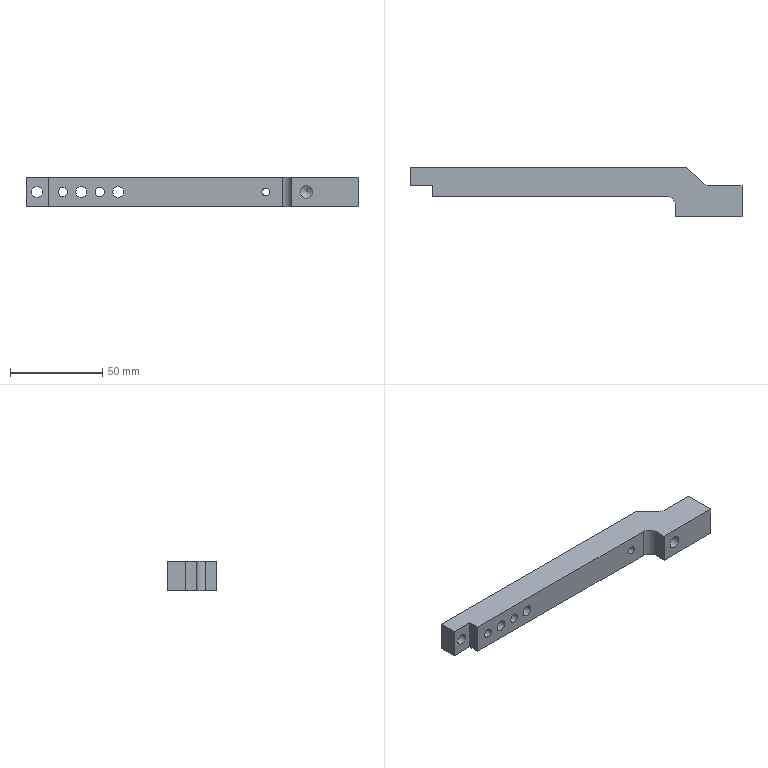Part | NX | features BREP 1 | 1 solid | 24 faces | box 180 x 27 x 16 mm | volume 43837 mm3 | plane 12 | cylinder 10 | cone 2 | commonest cylinder face diameters 6 x3 5 x2 6.8 x2 10 x2 4.2 x1
STEP:
#1=CARTESIAN_POINT('',(0.,6.,8.));
#2=VERTEX_POINT('',#1);
#3=CARTESIAN_POINT('',(0.,6.,-8.));
#4=VERTEX_POINT('',#3);
#5=CARTESIAN_POINT('',(0.,6.,8.));
#6=DIRECTION('',(0.,0.,-1.));
#7=VECTOR('',#6,1000.);
#8=LINE('',#5,#7);
#9=EDGE_CURVE('',#2,#4,#8,.T.);
#10=ORIENTED_EDGE('',*,*,#9,.F.);
#11=CARTESIAN_POINT('',(0.,16.,8.));
#12=VERTEX_POINT('',#11);
#13=CARTESIAN_POINT('',(0.,16.,8.));
#14=DIRECTION('',(0.,-1.,0.));
#15=VECTOR('',#14,1000.);
#16=LINE('',#13,#15);
#17=EDGE_CURVE('',#12,#2,#16,.T.);
#18=ORIENTED_EDGE('',*,*,#17,.F.);
#19=CARTESIAN_POINT('',(0.,16.,-8.));
#20=VERTEX_POINT('',#19);
#21=CARTESIAN_POINT('',(0.,16.,8.));
#22=DIRECTION('',(0.,0.,-1.));
#23=VECTOR('',#22,1000.);
#24=LINE('',#21,#23);
#25=EDGE_CURVE('',#12,#20,#24,.T.);
#26=ORIENTED_EDGE('',*,*,#25,.T.);
#27=CARTESIAN_POINT('',(0.,16.,-8.));
#28=DIRECTION('',(0.,-1.,0.));
#29=VECTOR('',#28,1000.);
#30=LINE('',#27,#29);
#31=EDGE_CURVE('',#20,#4,#30,.T.);
#32=ORIENTED_EDGE('',*,*,#31,.T.);
#33=EDGE_LOOP('',(#10,#18,#26,#32));
#34=FACE_BOUND('',#33,.T.);
#35=CARTESIAN_POINT('',(0.,16.,8.));
#36=DIRECTION('',(1.,0.,0.));
#37=DIRECTION('',(0.,0.,1.));
#38=AXIS2_PLACEMENT_3D('',#35,#36,#37);
#39=PLANE('',#38);
#40=ADVANCED_FACE('',(#34),#39,.F.);
#41=CARTESIAN_POINT('',(130.,0.,2.1));
#42=VERTEX_POINT('',#41);
#43=CARTESIAN_POINT('',(130.,0.,0.));
#44=DIRECTION('',(0.,1.,0.));
#45=DIRECTION('',(0.,0.,1.));
#46=AXIS2_PLACEMENT_3D('',#43,#44,#45);
#47=CIRCLE('',#46,2.1);
#48=EDGE_CURVE('',#42,#42,#47,.T.);
#49=ORIENTED_EDGE('',*,*,#48,.T.);
#50=EDGE_LOOP('',(#49));
#51=FACE_BOUND('',#50,.T.);
#52=CARTESIAN_POINT('',(40.,0.,2.5));
#53=VERTEX_POINT('',#52);
#54=CARTESIAN_POINT('',(40.,0.,0.));
#55=DIRECTION('',(0.,1.,0.));
#56=DIRECTION('',(0.,0.,1.));
#57=AXIS2_PLACEMENT_3D('',#54,#55,#56);
#58=CIRCLE('',#57,2.5);
#59=EDGE_CURVE('',#53,#53,#58,.T.);
#60=ORIENTED_EDGE('',*,*,#59,.T.);
#61=EDGE_LOOP('',(#60));
#62=FACE_BOUND('',#61,.T.);
#63=CARTESIAN_POINT('',(20.,0.,2.5));
#64=VERTEX_POINT('',#63);
#65=CARTESIAN_POINT('',(20.,0.,0.));
#66=DIRECTION('',(0.,1.,0.));
#67=DIRECTION('',(0.,0.,1.));
#68=AXIS2_PLACEMENT_3D('',#65,#66,#67);
#69=CIRCLE('',#68,2.5);
#70=EDGE_CURVE('',#64,#64,#69,.T.);
#71=ORIENTED_EDGE('',*,*,#70,.T.);
#72=EDGE_LOOP('',(#71));
#73=FACE_BOUND('',#72,.T.);
#74=CARTESIAN_POINT('',(50.,0.,3.));
#75=VERTEX_POINT('',#74);
#76=CARTESIAN_POINT('',(50.,0.,0.));
#77=DIRECTION('',(0.,1.,0.));
#78=DIRECTION('',(0.,0.,1.));
#79=AXIS2_PLACEMENT_3D('',#76,#77,#78);
#80=CIRCLE('',#79,3.);
#81=EDGE_CURVE('',#75,#75,#80,.T.);
#82=ORIENTED_EDGE('',*,*,#81,.T.);
#83=EDGE_LOOP('',(#82));
#84=FACE_BOUND('',#83,.T.);
#85=CARTESIAN_POINT('',(30.,0.,3.));
#86=VERTEX_POINT('',#85);
#87=CARTESIAN_POINT('',(30.,0.,0.));
#88=DIRECTION('',(0.,1.,0.));
#89=DIRECTION('',(0.,0.,1.));
#90=AXIS2_PLACEMENT_3D('',#87,#88,#89);
#91=CIRCLE('',#90,3.);
#92=EDGE_CURVE('',#86,#86,#91,.T.);
#93=ORIENTED_EDGE('',*,*,#92,.T.);
#94=EDGE_LOOP('',(#93));
#95=FACE_BOUND('',#94,.T.);
#96=CARTESIAN_POINT('',(12.,0.,-8.));
#97=VERTEX_POINT('',#96);
#98=CARTESIAN_POINT('',(139.,0.,-8.));
#99=VERTEX_POINT('',#98);
#100=CARTESIAN_POINT('',(0.,0.,-8.));
#101=DIRECTION('',(1.,0.,0.));
#102=VECTOR('',#101,1000.);
#103=LINE('',#100,#102);
#104=EDGE_CURVE('',#97,#99,#103,.T.);
#105=ORIENTED_EDGE('',*,*,#104,.T.);
#106=CARTESIAN_POINT('',(139.,0.,8.));
#107=VERTEX_POINT('',#106);
#108=CARTESIAN_POINT('',(139.,0.,8.));
#109=DIRECTION('',(0.,0.,1.));
#110=VECTOR('',#109,1000.);
#111=LINE('',#108,#110);
#112=EDGE_CURVE('',#99,#107,#111,.T.);
#113=ORIENTED_EDGE('',*,*,#112,.T.);
#114=CARTESIAN_POINT('',(12.,0.,8.));
#115=VERTEX_POINT('',#114);
#116=CARTESIAN_POINT('',(0.,0.,8.));
#117=DIRECTION('',(1.,0.,0.));
#118=VECTOR('',#117,1000.);
#119=LINE('',#116,#118);
#120=EDGE_CURVE('',#115,#107,#119,.T.);
#121=ORIENTED_EDGE('',*,*,#120,.F.);
#122=CARTESIAN_POINT('',(12.,0.,-8.));
#123=DIRECTION('',(0.,0.,1.));
#124=VECTOR('',#123,1000.);
#125=LINE('',#122,#124);
#126=EDGE_CURVE('',#97,#115,#125,.T.);
#127=ORIENTED_EDGE('',*,*,#126,.F.);
#128=EDGE_LOOP('',(#105,#113,#121,#127));
#129=FACE_BOUND('',#128,.T.);
#130=CARTESIAN_POINT('',(0.,0.,8.));
#131=DIRECTION('',(0.,1.,0.));
#132=DIRECTION('',(0.,0.,-1.));
#133=AXIS2_PLACEMENT_3D('',#130,#131,#132);
#134=PLANE('',#133);
#135=ADVANCED_FACE('',(#51,#62,#73,#84,#95,#129),#134,.F.);
#136=CARTESIAN_POINT('',(144.,-5.,8.));
#137=VERTEX_POINT('',#136);
#138=CARTESIAN_POINT('',(144.,-11.,8.));
#139=VERTEX_POINT('',#138);
#140=CARTESIAN_POINT('',(144.,0.,8.));
#141=DIRECTION('',(0.,-1.,0.));
#142=VECTOR('',#141,1000.);
#143=LINE('',#140,#142);
#144=EDGE_CURVE('',#137,#139,#143,.T.);
#145=ORIENTED_EDGE('',*,*,#144,.F.);
#146=CARTESIAN_POINT('',(144.,-5.,-8.));
#147=VERTEX_POINT('',#146);
#148=CARTESIAN_POINT('',(144.,-5.,-8.));
#149=DIRECTION('',(0.,0.,-1.));
#150=VECTOR('',#149,1000.);
#151=LINE('',#148,#150);
#152=EDGE_CURVE('',#137,#147,#151,.T.);
#153=ORIENTED_EDGE('',*,*,#152,.T.);
#154=CARTESIAN_POINT('',(144.,-11.,-8.));
#155=VERTEX_POINT('',#154);
#156=CARTESIAN_POINT('',(144.,0.,-8.));
#157=DIRECTION('',(0.,-1.,0.));
#158=VECTOR('',#157,1000.);
#159=LINE('',#156,#158);
#160=EDGE_CURVE('',#147,#155,#159,.T.);
#161=ORIENTED_EDGE('',*,*,#160,.T.);
#162=CARTESIAN_POINT('',(144.,-11.,8.));
#163=DIRECTION('',(0.,0.,-1.));
#164=VECTOR('',#163,1000.);
#165=LINE('',#162,#164);
#166=EDGE_CURVE('',#139,#155,#165,.T.);
#167=ORIENTED_EDGE('',*,*,#166,.F.);
#168=EDGE_LOOP('',(#145,#153,#161,#167));
#169=FACE_BOUND('',#168,.T.);
#170=CARTESIAN_POINT('',(144.,0.,8.));
#171=DIRECTION('',(1.,0.,0.));
#172=DIRECTION('',(0.,0.,1.));
#173=AXIS2_PLACEMENT_3D('',#170,#171,#172);
#174=PLANE('',#173);
#175=ADVANCED_FACE('',(#169),#174,.F.);
#176=CARTESIAN_POINT('',(152.,-11.,-3.4));
#177=VERTEX_POINT('',#176);
#178=CARTESIAN_POINT('',(152.,-11.,0.));
#179=DIRECTION('',(0.,-1.,0.));
#180=DIRECTION('',(0.,0.,-1.));
#181=AXIS2_PLACEMENT_3D('',#178,#179,#180);
#182=CIRCLE('',#181,3.4);
#183=EDGE_CURVE('',#177,#177,#182,.T.);
#184=ORIENTED_EDGE('',*,*,#183,.F.);
#185=EDGE_LOOP('',(#184));
#186=FACE_BOUND('',#185,.T.);
#187=CARTESIAN_POINT('',(180.,-11.,-8.));
#188=VERTEX_POINT('',#187);
#189=CARTESIAN_POINT('',(144.,-11.,-8.));
#190=DIRECTION('',(1.,0.,0.));
#191=VECTOR('',#190,1000.);
#192=LINE('',#189,#191);
#193=EDGE_CURVE('',#155,#188,#192,.T.);
#194=ORIENTED_EDGE('',*,*,#193,.T.);
#195=CARTESIAN_POINT('',(180.,-11.,8.));
#196=VERTEX_POINT('',#195);
#197=CARTESIAN_POINT('',(180.,-11.,-8.));
#198=DIRECTION('',(0.,0.,1.));
#199=VECTOR('',#198,1000.);
#200=LINE('',#197,#199);
#201=EDGE_CURVE('',#188,#196,#200,.T.);
#202=ORIENTED_EDGE('',*,*,#201,.T.);
#203=CARTESIAN_POINT('',(144.,-11.,8.));
#204=DIRECTION('',(1.,0.,0.));
#205=VECTOR('',#204,1000.);
#206=LINE('',#203,#205);
#207=EDGE_CURVE('',#139,#196,#206,.T.);
#208=ORIENTED_EDGE('',*,*,#207,.F.);
#209=ORIENTED_EDGE('',*,*,#166,.T.);
#210=EDGE_LOOP('',(#194,#202,#208,#209));
#211=FACE_BOUND('',#210,.T.);
#212=CARTESIAN_POINT('',(144.,-11.,8.));
#213=DIRECTION('',(0.,1.,0.));
#214=DIRECTION('',(0.,0.,-1.));
#215=AXIS2_PLACEMENT_3D('',#212,#213,#214);
#216=PLANE('',#215);
#217=ADVANCED_FACE('',(#186,#211),#216,.F.);
#218=CARTESIAN_POINT('',(158.536,7.464,8.));
#219=VERTEX_POINT('',#218);
#220=CARTESIAN_POINT('',(150.,16.,8.));
#221=VERTEX_POINT('',#220);
#222=CARTESIAN_POINT('',(160.,6.,8.));
#223=DIRECTION('',(-0.7071,0.7071,0.));
#224=VECTOR('',#223,1000.);
#225=LINE('',#222,#224);
#226=EDGE_CURVE('',#219,#221,#225,.T.);
#227=ORIENTED_EDGE('',*,*,#226,.F.);
#228=CARTESIAN_POINT('',(158.536,7.464,-8.));
#229=VERTEX_POINT('',#228);
#230=CARTESIAN_POINT('',(158.536,7.464,8.));
#231=DIRECTION('',(0.,0.,-1.));
#232=VECTOR('',#231,1000.);
#233=LINE('',#230,#232);
#234=EDGE_CURVE('',#219,#229,#233,.T.);
#235=ORIENTED_EDGE('',*,*,#234,.T.);
#236=CARTESIAN_POINT('',(150.,16.,-8.));
#237=VERTEX_POINT('',#236);
#238=CARTESIAN_POINT('',(160.,6.,-8.));
#239=DIRECTION('',(-0.7071,0.7071,0.));
#240=VECTOR('',#239,1000.);
#241=LINE('',#238,#240);
#242=EDGE_CURVE('',#229,#237,#241,.T.);
#243=ORIENTED_EDGE('',*,*,#242,.T.);
#244=CARTESIAN_POINT('',(150.,16.,8.));
#245=DIRECTION('',(0.,0.,-1.));
#246=VECTOR('',#245,1000.);
#247=LINE('',#244,#246);
#248=EDGE_CURVE('',#221,#237,#247,.T.);
#249=ORIENTED_EDGE('',*,*,#248,.F.);
#250=EDGE_LOOP('',(#227,#235,#243,#249));
#251=FACE_BOUND('',#250,.T.);
#252=CARTESIAN_POINT('',(160.,6.,8.));
#253=DIRECTION('',(-0.7071,-0.7071,0.));
#254=DIRECTION('',(-0.7071,0.7071,0.));
#255=AXIS2_PLACEMENT_3D('',#252,#253,#254);
#256=PLANE('',#255);
#257=ADVANCED_FACE('',(#251),#256,.F.);
#258=CARTESIAN_POINT('',(130.,16.,2.1));
#259=VERTEX_POINT('',#258);
#260=CARTESIAN_POINT('',(130.,16.,0.));
#261=DIRECTION('',(0.,1.,0.));
#262=DIRECTION('',(0.,0.,1.));
#263=AXIS2_PLACEMENT_3D('',#260,#261,#262);
#264=CIRCLE('',#263,2.1);
#265=EDGE_CURVE('',#259,#259,#264,.T.);
#266=ORIENTED_EDGE('',*,*,#265,.F.);
#267=EDGE_LOOP('',(#266));
#268=FACE_BOUND('',#267,.T.);
#269=CARTESIAN_POINT('',(40.,16.,2.5));
#270=VERTEX_POINT('',#269);
#271=CARTESIAN_POINT('',(40.,16.,0.));
#272=DIRECTION('',(0.,1.,0.));
#273=DIRECTION('',(0.,0.,1.));
#274=AXIS2_PLACEMENT_3D('',#271,#272,#273);
#275=CIRCLE('',#274,2.5);
#276=EDGE_CURVE('',#270,#270,#275,.T.);
#277=ORIENTED_EDGE('',*,*,#276,.F.);
#278=EDGE_LOOP('',(#277));
#279=FACE_BOUND('',#278,.T.);
#280=CARTESIAN_POINT('',(20.,16.,2.5));
#281=VERTEX_POINT('',#280);
#282=CARTESIAN_POINT('',(20.,16.,0.));
#283=DIRECTION('',(0.,1.,0.));
#284=DIRECTION('',(0.,0.,1.));
#285=AXIS2_PLACEMENT_3D('',#282,#283,#284);
#286=CIRCLE('',#285,2.5);
#287=EDGE_CURVE('',#281,#281,#286,.T.);
#288=ORIENTED_EDGE('',*,*,#287,.F.);
#289=EDGE_LOOP('',(#288));
#290=FACE_BOUND('',#289,.T.);
#291=CARTESIAN_POINT('',(50.,16.,3.));
#292=VERTEX_POINT('',#291);
#293=CARTESIAN_POINT('',(50.,16.,0.));
#294=DIRECTION('',(0.,1.,0.));
#295=DIRECTION('',(0.,0.,1.));
#296=AXIS2_PLACEMENT_3D('',#293,#294,#295);
#297=CIRCLE('',#296,3.);
#298=EDGE_CURVE('',#292,#292,#297,.T.);
#299=ORIENTED_EDGE('',*,*,#298,.F.);
#300=EDGE_LOOP('',(#299));
#301=FACE_BOUND('',#300,.T.);
#302=CARTESIAN_POINT('',(30.,16.,3.));
#303=VERTEX_POINT('',#302);
#304=CARTESIAN_POINT('',(30.,16.,0.));
#305=DIRECTION('',(0.,1.,0.));
#306=DIRECTION('',(0.,0.,1.));
#307=AXIS2_PLACEMENT_3D('',#304,#305,#306);
#308=CIRCLE('',#307,3.);
#309=EDGE_CURVE('',#303,#303,#308,.T.);
#310=ORIENTED_EDGE('',*,*,#309,.F.);
#311=EDGE_LOOP('',(#310));
#312=FACE_BOUND('',#311,.T.);
#313=CARTESIAN_POINT('',(6.,16.,-3.));
#314=VERTEX_POINT('',#313);
#315=CARTESIAN_POINT('',(6.,16.,0.));
#316=DIRECTION('',(0.,-1.,0.));
#317=DIRECTION('',(0.,0.,-1.));
#318=AXIS2_PLACEMENT_3D('',#315,#316,#317);
#319=CIRCLE('',#318,3.);
#320=EDGE_CURVE('',#314,#314,#319,.T.);
#321=ORIENTED_EDGE('',*,*,#320,.T.);
#322=EDGE_LOOP('',(#321));
#323=FACE_BOUND('',#322,.T.);
#324=CARTESIAN_POINT('',(150.,16.,-8.));
#325=DIRECTION('',(-1.,0.,0.));
#326=VECTOR('',#325,1000.);
#327=LINE('',#324,#326);
#328=EDGE_CURVE('',#237,#20,#327,.T.);
#329=ORIENTED_EDGE('',*,*,#328,.T.);
#330=ORIENTED_EDGE('',*,*,#25,.F.);
#331=CARTESIAN_POINT('',(150.,16.,8.));
#332=DIRECTION('',(-1.,0.,0.));
#333=VECTOR('',#332,1000.);
#334=LINE('',#331,#333);
#335=EDGE_CURVE('',#221,#12,#334,.T.);
#336=ORIENTED_EDGE('',*,*,#335,.F.);
#337=ORIENTED_EDGE('',*,*,#248,.T.);
#338=EDGE_LOOP('',(#329,#330,#336,#337));
#339=FACE_BOUND('',#338,.T.);
#340=CARTESIAN_POINT('',(150.,16.,8.));
#341=DIRECTION('',(0.,-1.,0.));
#342=DIRECTION('',(-1.,0.,0.));
#343=AXIS2_PLACEMENT_3D('',#340,#341,#342);
#344=PLANE('',#343);
#345=ADVANCED_FACE('',(#268,#279,#290,#301,#312,#323,#339),#344,.F.);
#346=CARTESIAN_POINT('',(12.,6.,8.));
#347=VERTEX_POINT('',#346);
#348=CARTESIAN_POINT('',(12.,6.,8.));
#349=DIRECTION('',(0.,-1.,0.));
#350=VECTOR('',#349,1000.);
#351=LINE('',#348,#350);
#352=EDGE_CURVE('',#347,#115,#351,.T.);
#353=ORIENTED_EDGE('',*,*,#352,.T.);
#354=ORIENTED_EDGE('',*,*,#120,.T.);
#355=CARTESIAN_POINT('',(139.,-5.,8.));
#356=DIRECTION('',(0.,0.,-1.));
#357=DIRECTION('',(1.,0.,0.));
#358=AXIS2_PLACEMENT_3D('',#355,#356,#357);
#359=CIRCLE('',#358,5.);
#360=EDGE_CURVE('',#107,#137,#359,.T.);
#361=ORIENTED_EDGE('',*,*,#360,.T.);
#362=ORIENTED_EDGE('',*,*,#144,.T.);
#363=ORIENTED_EDGE('',*,*,#207,.T.);
#364=CARTESIAN_POINT('',(180.,6.,8.));
#365=VERTEX_POINT('',#364);
#366=CARTESIAN_POINT('',(180.,6.,8.));
#367=DIRECTION('',(0.,1.,0.));
#368=VECTOR('',#367,1000.);
#369=LINE('',#366,#368);
#370=EDGE_CURVE('',#196,#365,#369,.T.);
#371=ORIENTED_EDGE('',*,*,#370,.T.);
#372=CARTESIAN_POINT('',(162.071,6.,8.));
#373=VERTEX_POINT('',#372);
#374=CARTESIAN_POINT('',(160.,6.,8.));
#375=DIRECTION('',(-1.,0.,0.));
#376=VECTOR('',#375,1000.);
#377=LINE('',#374,#376);
#378=EDGE_CURVE('',#365,#373,#377,.T.);
#379=ORIENTED_EDGE('',*,*,#378,.T.);
#380=CARTESIAN_POINT('',(162.071,11.,8.));
#381=DIRECTION('',(0.,0.,-1.));
#382=DIRECTION('',(1.,0.,0.));
#383=AXIS2_PLACEMENT_3D('',#380,#381,#382);
#384=CIRCLE('',#383,5.);
#385=EDGE_CURVE('',#373,#219,#384,.T.);
#386=ORIENTED_EDGE('',*,*,#385,.T.);
#387=ORIENTED_EDGE('',*,*,#226,.T.);
#388=ORIENTED_EDGE('',*,*,#335,.T.);
#389=ORIENTED_EDGE('',*,*,#17,.T.);
#390=CARTESIAN_POINT('',(12.,6.,8.));
#391=DIRECTION('',(-1.,0.,0.));
#392=VECTOR('',#391,1000.);
#393=LINE('',#390,#392);
#394=EDGE_CURVE('',#347,#2,#393,.T.);
#395=ORIENTED_EDGE('',*,*,#394,.F.);
#396=EDGE_LOOP('',(#353,#354,#361,#362,#363,#371,#379,#386,#387,#388,#389,#395));
#397=FACE_BOUND('',#396,.T.);
#398=CARTESIAN_POINT('',(0.,0.,8.));
#399=DIRECTION('',(0.,0.,1.));
#400=DIRECTION('',(-1.,0.,0.));
#401=AXIS2_PLACEMENT_3D('',#398,#399,#400);
#402=PLANE('',#401);
#403=ADVANCED_FACE('',(#397),#402,.T.);
#404=ORIENTED_EDGE('',*,*,#104,.F.);
#405=CARTESIAN_POINT('',(12.,6.,-8.));
#406=VERTEX_POINT('',#405);
#407=CARTESIAN_POINT('',(12.,6.,-8.));
#408=DIRECTION('',(0.,-1.,0.));
#409=VECTOR('',#408,1000.);
#410=LINE('',#407,#409);
#411=EDGE_CURVE('',#406,#97,#410,.T.);
#412=ORIENTED_EDGE('',*,*,#411,.F.);
#413=CARTESIAN_POINT('',(0.,6.,-8.));
#414=DIRECTION('',(1.,0.,0.));
#415=VECTOR('',#414,1000.);
#416=LINE('',#413,#415);
#417=EDGE_CURVE('',#4,#406,#416,.T.);
#418=ORIENTED_EDGE('',*,*,#417,.F.);
#419=ORIENTED_EDGE('',*,*,#31,.F.);
#420=ORIENTED_EDGE('',*,*,#328,.F.);
#421=ORIENTED_EDGE('',*,*,#242,.F.);
#422=CARTESIAN_POINT('',(162.071,6.,-8.));
#423=VERTEX_POINT('',#422);
#424=CARTESIAN_POINT('',(162.071,11.,-8.));
#425=DIRECTION('',(0.,0.,1.));
#426=DIRECTION('',(1.,0.,0.));
#427=AXIS2_PLACEMENT_3D('',#424,#425,#426);
#428=CIRCLE('',#427,5.);
#429=EDGE_CURVE('',#229,#423,#428,.T.);
#430=ORIENTED_EDGE('',*,*,#429,.T.);
#431=CARTESIAN_POINT('',(180.,6.,-8.));
#432=VERTEX_POINT('',#431);
#433=CARTESIAN_POINT('',(160.,6.,-8.));
#434=DIRECTION('',(-1.,0.,0.));
#435=VECTOR('',#434,1000.);
#436=LINE('',#433,#435);
#437=EDGE_CURVE('',#432,#423,#436,.T.);
#438=ORIENTED_EDGE('',*,*,#437,.F.);
#439=CARTESIAN_POINT('',(180.,6.,-8.));
#440=DIRECTION('',(0.,1.,0.));
#441=VECTOR('',#440,1000.);
#442=LINE('',#439,#441);
#443=EDGE_CURVE('',#188,#432,#442,.T.);
#444=ORIENTED_EDGE('',*,*,#443,.F.);
#445=ORIENTED_EDGE('',*,*,#193,.F.);
#446=ORIENTED_EDGE('',*,*,#160,.F.);
#447=CARTESIAN_POINT('',(139.,-5.,-8.));
#448=DIRECTION('',(0.,0.,1.));
#449=DIRECTION('',(1.,0.,0.));
#450=AXIS2_PLACEMENT_3D('',#447,#448,#449);
#451=CIRCLE('',#450,5.);
#452=EDGE_CURVE('',#147,#99,#451,.T.);
#453=ORIENTED_EDGE('',*,*,#452,.T.);
#454=EDGE_LOOP('',(#404,#412,#418,#419,#420,#421,#430,#438,#444,#445,#446,#453));
#455=FACE_BOUND('',#454,.T.);
#456=CARTESIAN_POINT('',(0.,0.,-8.));
#457=DIRECTION('',(0.,0.,1.));
#458=DIRECTION('',(-1.,0.,0.));
#459=AXIS2_PLACEMENT_3D('',#456,#457,#458);
#460=PLANE('',#459);
#461=ADVANCED_FACE('',(#455),#460,.F.);
#462=ORIENTED_EDGE('',*,*,#126,.T.);
#463=ORIENTED_EDGE('',*,*,#352,.F.);
#464=CARTESIAN_POINT('',(12.,6.,-8.));
#465=DIRECTION('',(0.,0.,1.));
#466=VECTOR('',#465,1000.);
#467=LINE('',#464,#466);
#468=EDGE_CURVE('',#406,#347,#467,.T.);
#469=ORIENTED_EDGE('',*,*,#468,.F.);
#470=ORIENTED_EDGE('',*,*,#411,.T.);
#471=EDGE_LOOP('',(#462,#463,#469,#470));
#472=FACE_BOUND('',#471,.T.);
#473=CARTESIAN_POINT('',(12.,6.,-8.));
#474=DIRECTION('',(1.,0.,0.));
#475=DIRECTION('',(0.,0.,1.));
#476=AXIS2_PLACEMENT_3D('',#473,#474,#475);
#477=PLANE('',#476);
#478=ADVANCED_FACE('',(#472),#477,.F.);
#479=CARTESIAN_POINT('',(6.,6.,-3.));
#480=VERTEX_POINT('',#479);
#481=CARTESIAN_POINT('',(6.,6.,0.));
#482=DIRECTION('',(0.,-1.,0.));
#483=DIRECTION('',(0.,0.,-1.));
#484=AXIS2_PLACEMENT_3D('',#481,#482,#483);
#485=CIRCLE('',#484,3.);
#486=EDGE_CURVE('',#480,#480,#485,.T.);
#487=ORIENTED_EDGE('',*,*,#486,.F.);
#488=EDGE_LOOP('',(#487));
#489=FACE_BOUND('',#488,.T.);
#490=ORIENTED_EDGE('',*,*,#394,.T.);
#491=ORIENTED_EDGE('',*,*,#9,.T.);
#492=ORIENTED_EDGE('',*,*,#417,.T.);
#493=ORIENTED_EDGE('',*,*,#468,.T.);
#494=EDGE_LOOP('',(#490,#491,#492,#493));
#495=FACE_BOUND('',#494,.T.);
#496=CARTESIAN_POINT('',(0.,6.,0.));
#497=DIRECTION('',(0.,-1.,0.));
#498=DIRECTION('',(0.,0.,1.));
#499=AXIS2_PLACEMENT_3D('',#496,#497,#498);
#500=PLANE('',#499);
#501=ADVANCED_FACE('',(#489,#495),#500,.T.);
#502=ORIENTED_EDGE('',*,*,#320,.F.);
#503=EDGE_LOOP('',(#502));
#504=FACE_BOUND('',#503,.T.);
#505=ORIENTED_EDGE('',*,*,#486,.T.);
#506=EDGE_LOOP('',(#505));
#507=FACE_BOUND('',#506,.T.);
#508=CARTESIAN_POINT('',(6.,6.,0.));
#509=DIRECTION('',(0.,-1.,0.));
#510=DIRECTION('',(0.,0.,1.));
#511=AXIS2_PLACEMENT_3D('',#508,#509,#510);
#512=CYLINDRICAL_SURFACE('',#511,3.);
#513=ADVANCED_FACE('',(#504,#507),#512,.F.);
#514=ORIENTED_EDGE('',*,*,#360,.F.);
#515=ORIENTED_EDGE('',*,*,#112,.F.);
#516=ORIENTED_EDGE('',*,*,#452,.F.);
#517=ORIENTED_EDGE('',*,*,#152,.F.);
#518=EDGE_LOOP('',(#514,#515,#516,#517));
#519=FACE_BOUND('',#518,.T.);
#520=CARTESIAN_POINT('',(139.,-5.,8.));
#521=DIRECTION('',(0.,0.,1.));
#522=DIRECTION('',(-1.,0.,0.));
#523=AXIS2_PLACEMENT_3D('',#520,#521,#522);
#524=CYLINDRICAL_SURFACE('',#523,5.);
#525=ADVANCED_FACE('',(#519),#524,.F.);
#526=CARTESIAN_POINT('',(152.,10.793,0.));
#527=VERTEX_POINT('',#526);
#528=VERTEX_LOOP('',#527);
#529=FACE_BOUND('',#528,.T.);
#530=CARTESIAN_POINT('',(152.,8.75,-3.4));
#531=VERTEX_POINT('',#530);
#532=CARTESIAN_POINT('',(152.,8.75,0.));
#533=DIRECTION('',(0.,-1.,0.));
#534=DIRECTION('',(0.,0.,-1.));
#535=AXIS2_PLACEMENT_3D('',#532,#533,#534);
#536=CIRCLE('',#535,3.4);
#537=EDGE_CURVE('',#531,#531,#536,.T.);
#538=ORIENTED_EDGE('',*,*,#537,.T.);
#539=EDGE_LOOP('',(#538));
#540=FACE_BOUND('',#539,.T.);
#541=CARTESIAN_POINT('',(152.,8.75,0.));
#542=DIRECTION('',(0.,-1.,0.));
#543=DIRECTION('',(0.,0.,1.));
#544=AXIS2_PLACEMENT_3D('',#541,#542,#543);
#545=CONICAL_SURFACE('',#544,3.4,1.03);
#546=ADVANCED_FACE('',(#529,#540),#545,.F.);
#547=ORIENTED_EDGE('',*,*,#537,.F.);
#548=EDGE_LOOP('',(#547));
#549=FACE_BOUND('',#548,.T.);
#550=ORIENTED_EDGE('',*,*,#183,.T.);
#551=EDGE_LOOP('',(#550));
#552=FACE_BOUND('',#551,.T.);
#553=CARTESIAN_POINT('',(152.,-11.,0.));
#554=DIRECTION('',(0.,-1.,0.));
#555=DIRECTION('',(0.,0.,1.));
#556=AXIS2_PLACEMENT_3D('',#553,#554,#555);
#557=CYLINDRICAL_SURFACE('',#556,3.4);
#558=ADVANCED_FACE('',(#549,#552),#557,.F.);
#559=ORIENTED_EDGE('',*,*,#309,.T.);
#560=EDGE_LOOP('',(#559));
#561=FACE_BOUND('',#560,.T.);
#562=ORIENTED_EDGE('',*,*,#92,.F.);
#563=EDGE_LOOP('',(#562));
#564=FACE_BOUND('',#563,.T.);
#565=CARTESIAN_POINT('',(30.,16.,0.));
#566=DIRECTION('',(0.,1.,0.));
#567=DIRECTION('',(0.,0.,-1.));
#568=AXIS2_PLACEMENT_3D('',#565,#566,#567);
#569=CYLINDRICAL_SURFACE('',#568,3.);
#570=ADVANCED_FACE('',(#561,#564),#569,.F.);
#571=ORIENTED_EDGE('',*,*,#298,.T.);
#572=EDGE_LOOP('',(#571));
#573=FACE_BOUND('',#572,.T.);
#574=ORIENTED_EDGE('',*,*,#81,.F.);
#575=EDGE_LOOP('',(#574));
#576=FACE_BOUND('',#575,.T.);
#577=CARTESIAN_POINT('',(50.,16.,0.));
#578=DIRECTION('',(0.,1.,0.));
#579=DIRECTION('',(0.,0.,-1.));
#580=AXIS2_PLACEMENT_3D('',#577,#578,#579);
#581=CYLINDRICAL_SURFACE('',#580,3.);
#582=ADVANCED_FACE('',(#573,#576),#581,.F.);
#583=ORIENTED_EDGE('',*,*,#287,.T.);
#584=EDGE_LOOP('',(#583));
#585=FACE_BOUND('',#584,.T.);
#586=ORIENTED_EDGE('',*,*,#70,.F.);
#587=EDGE_LOOP('',(#586));
#588=FACE_BOUND('',#587,.T.);
#589=CARTESIAN_POINT('',(20.,16.,0.));
#590=DIRECTION('',(0.,1.,0.));
#591=DIRECTION('',(0.,0.,-1.));
#592=AXIS2_PLACEMENT_3D('',#589,#590,#591);
#593=CYLINDRICAL_SURFACE('',#592,2.5);
#594=ADVANCED_FACE('',(#585,#588),#593,.F.);
#595=ORIENTED_EDGE('',*,*,#276,.T.);
#596=EDGE_LOOP('',(#595));
#597=FACE_BOUND('',#596,.T.);
#598=ORIENTED_EDGE('',*,*,#59,.F.);
#599=EDGE_LOOP('',(#598));
#600=FACE_BOUND('',#599,.T.);
#601=CARTESIAN_POINT('',(40.,16.,0.));
#602=DIRECTION('',(0.,1.,0.));
#603=DIRECTION('',(0.,0.,-1.));
#604=AXIS2_PLACEMENT_3D('',#601,#602,#603);
#605=CYLINDRICAL_SURFACE('',#604,2.5);
#606=ADVANCED_FACE('',(#597,#600),#605,.F.);
#607=ORIENTED_EDGE('',*,*,#265,.T.);
#608=EDGE_LOOP('',(#607));
#609=FACE_BOUND('',#608,.T.);
#610=ORIENTED_EDGE('',*,*,#48,.F.);
#611=EDGE_LOOP('',(#610));
#612=FACE_BOUND('',#611,.T.);
#613=CARTESIAN_POINT('',(130.,16.,0.));
#614=DIRECTION('',(0.,1.,0.));
#615=DIRECTION('',(0.,0.,-1.));
#616=AXIS2_PLACEMENT_3D('',#613,#614,#615);
#617=CYLINDRICAL_SURFACE('',#616,2.1);
#618=ADVANCED_FACE('',(#609,#612),#617,.F.);
#619=ORIENTED_EDGE('',*,*,#437,.T.);
#620=CARTESIAN_POINT('',(162.071,6.,-8.));
#621=DIRECTION('',(0.,0.,1.));
#622=VECTOR('',#621,1000.);
#623=LINE('',#620,#622);
#624=EDGE_CURVE('',#423,#373,#623,.T.);
#625=ORIENTED_EDGE('',*,*,#624,.T.);
#626=ORIENTED_EDGE('',*,*,#378,.F.);
#627=CARTESIAN_POINT('',(180.,6.,-8.));
#628=DIRECTION('',(0.,0.,1.));
#629=VECTOR('',#628,1000.);
#630=LINE('',#627,#629);
#631=EDGE_CURVE('',#432,#365,#630,.T.);
#632=ORIENTED_EDGE('',*,*,#631,.F.);
#633=EDGE_LOOP('',(#619,#625,#626,#632));
#634=FACE_BOUND('',#633,.T.);
#635=CARTESIAN_POINT('',(160.,6.,-8.));
#636=DIRECTION('',(0.,1.,0.));
#637=DIRECTION('',(1.,0.,0.));
#638=AXIS2_PLACEMENT_3D('',#635,#636,#637);
#639=PLANE('',#638);
#640=ADVANCED_FACE('',(#634),#639,.T.);
#641=CARTESIAN_POINT('',(180.,-2.5,-3.4));
#642=VERTEX_POINT('',#641);
#643=CARTESIAN_POINT('',(180.,-2.5,0.));
#644=DIRECTION('',(1.,0.,0.));
#645=DIRECTION('',(0.,0.,-1.));
#646=AXIS2_PLACEMENT_3D('',#643,#644,#645);
#647=CIRCLE('',#646,3.4);
#648=EDGE_CURVE('',#642,#642,#647,.T.);
#649=ORIENTED_EDGE('',*,*,#648,.F.);
#650=EDGE_LOOP('',(#649));
#651=FACE_BOUND('',#650,.T.);
#652=ORIENTED_EDGE('',*,*,#370,.F.);
#653=ORIENTED_EDGE('',*,*,#201,.F.);
#654=ORIENTED_EDGE('',*,*,#443,.T.);
#655=ORIENTED_EDGE('',*,*,#631,.T.);
#656=EDGE_LOOP('',(#652,#653,#654,#655));
#657=FACE_BOUND('',#656,.T.);
#658=CARTESIAN_POINT('',(180.,6.,-8.));
#659=DIRECTION('',(1.,0.,0.));
#660=DIRECTION('',(0.,0.,1.));
#661=AXIS2_PLACEMENT_3D('',#658,#659,#660);
#662=PLANE('',#661);
#663=ADVANCED_FACE('',(#651,#657),#662,.T.);
#664=ORIENTED_EDGE('',*,*,#385,.F.);
#665=ORIENTED_EDGE('',*,*,#624,.F.);
#666=ORIENTED_EDGE('',*,*,#429,.F.);
#667=ORIENTED_EDGE('',*,*,#234,.F.);
#668=EDGE_LOOP('',(#664,#665,#666,#667));
#669=FACE_BOUND('',#668,.T.);
#670=CARTESIAN_POINT('',(162.071,11.,8.));
#671=DIRECTION('',(0.,0.,-1.));
#672=DIRECTION('',(1.,0.,0.));
#673=AXIS2_PLACEMENT_3D('',#670,#671,#672);
#674=CYLINDRICAL_SURFACE('',#673,5.);
#675=ADVANCED_FACE('',(#669),#674,.F.);
#676=CARTESIAN_POINT('',(158.207,-2.5,0.));
#677=VERTEX_POINT('',#676);
#678=VERTEX_LOOP('',#677);
#679=FACE_BOUND('',#678,.T.);
#680=CARTESIAN_POINT('',(160.25,-2.5,-3.4));
#681=VERTEX_POINT('',#680);
#682=CARTESIAN_POINT('',(160.25,-2.5,0.));
#683=DIRECTION('',(1.,0.,0.));
#684=DIRECTION('',(0.,0.,-1.));
#685=AXIS2_PLACEMENT_3D('',#682,#683,#684);
#686=CIRCLE('',#685,3.4);
#687=EDGE_CURVE('',#681,#681,#686,.T.);
#688=ORIENTED_EDGE('',*,*,#687,.T.);
#689=EDGE_LOOP('',(#688));
#690=FACE_BOUND('',#689,.T.);
#691=CARTESIAN_POINT('',(160.25,-2.5,0.));
#692=DIRECTION('',(1.,0.,0.));
#693=DIRECTION('',(0.,0.,1.));
#694=AXIS2_PLACEMENT_3D('',#691,#692,#693);
#695=CONICAL_SURFACE('',#694,3.4,1.03);
#696=ADVANCED_FACE('',(#679,#690),#695,.F.);
#697=ORIENTED_EDGE('',*,*,#687,.F.);
#698=EDGE_LOOP('',(#697));
#699=FACE_BOUND('',#698,.T.);
#700=ORIENTED_EDGE('',*,*,#648,.T.);
#701=EDGE_LOOP('',(#700));
#702=FACE_BOUND('',#701,.T.);
#703=CARTESIAN_POINT('',(180.,-2.5,0.));
#704=DIRECTION('',(1.,0.,0.));
#705=DIRECTION('',(0.,0.,1.));
#706=AXIS2_PLACEMENT_3D('',#703,#704,#705);
#707=CYLINDRICAL_SURFACE('',#706,3.4);
#708=ADVANCED_FACE('',(#699,#702),#707,.F.);
#709=CLOSED_SHELL('',(#40,#135,#175,#217,#257,#345,#403,#461,#478,#501,#513,#525,#546,#558,#570,#582,#594,#606,#618,#640,#663,#675,#696,#708));
#710=MANIFOLD_SOLID_BREP('',#709);
#711=(LENGTH_UNIT()NAMED_UNIT(*)SI_UNIT(.MILLI.,.METRE.));
#712=UNCERTAINTY_MEASURE_WITH_UNIT(LENGTH_MEASURE(0.00001),#711,'','');
#713=(NAMED_UNIT(*)PLANE_ANGLE_UNIT()SI_UNIT($,.RADIAN.));
#714=(NAMED_UNIT(*)SI_UNIT($,.STERADIAN.)SOLID_ANGLE_UNIT());
#715=(GEOMETRIC_REPRESENTATION_CONTEXT(3)GLOBAL_UNCERTAINTY_ASSIGNED_CONTEXT((#712))GLOBAL_UNIT_ASSIGNED_CONTEXT((#711,#713,#714))REPRESENTATION_CONTEXT('',''));
#716=ADVANCED_BREP_SHAPE_REPRESENTATION('',(#710),#715);